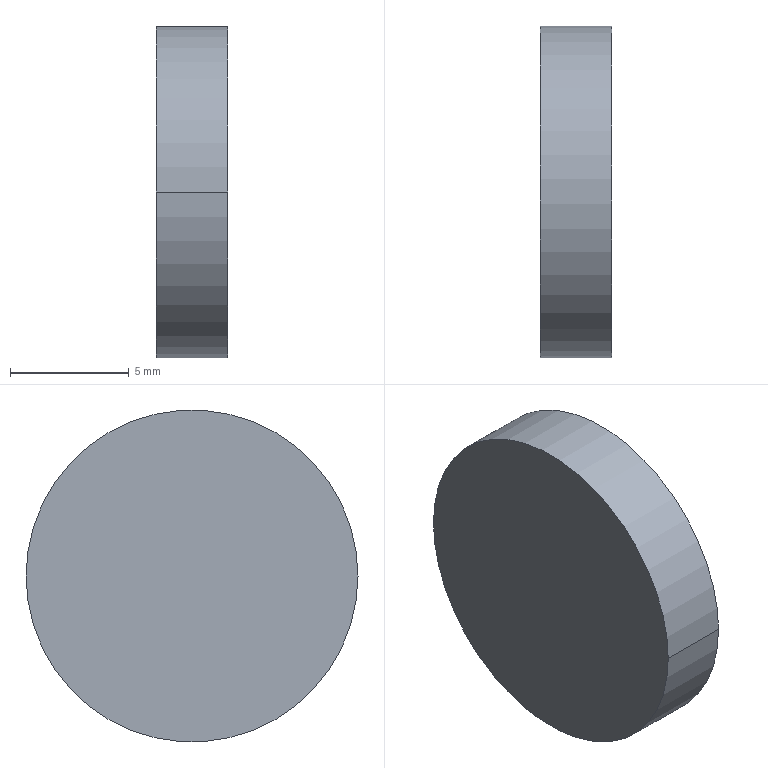Part | STEP file | LG-CAP_M8 | 1 solid | 4 faces | box 3 x 14 x 14 mm | volume 461.814 mm3 | cylinder 2 | plane 2 | commonest cylinder face diameters 14 x2
STEP:
#1=CARTESIAN_POINT('',(0.,0.,0.));
#2=DIRECTION('',(0.,0.,1.));
#3=DIRECTION('',(1.,0.,0.));
#4=AXIS2_PLACEMENT_3D('',#1,#2,#3);
#5=CARTESIAN_POINT('',(0.,-7.,0.));
#6=VERTEX_POINT('',#5);
#7=CARTESIAN_POINT('',(0.,7.,0.));
#8=VERTEX_POINT('',#7);
#9=CARTESIAN_POINT('',(0.,0.,0.));
#10=DIRECTION('',(1.,0.,0.));
#11=DIRECTION('',(0.,-1.,0.));
#12=AXIS2_PLACEMENT_3D('',#9,#10,#11);
#13=CIRCLE('',#12,7.);
#14=CARTESIAN_POINT('',(0.,0.,0.));
#15=DIRECTION('',(1.,0.,0.));
#16=DIRECTION('',(0.,-1.,0.));
#17=AXIS2_PLACEMENT_3D('',#14,#15,#16);
#18=CYLINDRICAL_SURFACE('',#17,7.);
#19=CARTESIAN_POINT('',(0.,0.));
#20=DIRECTION('',(1.,0.));
#21=VECTOR('',#20,1.);
#22=LINE('',#19,#21);
#23=(GEOMETRIC_REPRESENTATION_CONTEXT(2)PARAMETRIC_REPRESENTATION_CONTEXT()REPRESENTATION_CONTEXT('',''));
#24=DEFINITIONAL_REPRESENTATION('',(#22),#23);
#25=PCURVE('',#18,#24);
#26=CARTESIAN_POINT('',(0.,0.,0.));
#27=DIRECTION('',(-1.,0.,0.));
#28=DIRECTION('',(0.,1.,0.));
#29=AXIS2_PLACEMENT_3D('',#26,#27,#28);
#30=PLANE('',#29);
#31=CARTESIAN_POINT('',(-7.,0.));
#32=CARTESIAN_POINT('',(-7.,12.124));
#33=CARTESIAN_POINT('',(3.5,6.062));
#34=CARTESIAN_POINT('',(14.,0.));
#35=CARTESIAN_POINT('',(3.5,-6.062));
#36=CARTESIAN_POINT('',(-7.,-12.124));
#37=CARTESIAN_POINT('',(-7.,0.));
#38=(BOUNDED_CURVE()B_SPLINE_CURVE(2,(#31,#32,#33,#34,#35,#36,#37),.UNSPECIFIED.,.T.,.F.)B_SPLINE_CURVE_WITH_KNOTS((1,2,2,2,2,1),(-2.094,0.,2.094,4.189,6.283,8.378),.UNSPECIFIED.)CURVE()GEOMETRIC_REPRESENTATION_ITEM()RATIONAL_B_SPLINE_CURVE((1.,0.5,1.,0.5,1.,0.5,1.))REPRESENTATION_ITEM(''));
#39=(GEOMETRIC_REPRESENTATION_CONTEXT(2)PARAMETRIC_REPRESENTATION_CONTEXT()REPRESENTATION_CONTEXT('',''));
#40=DEFINITIONAL_REPRESENTATION('',(#38),#39);
#41=PCURVE('',#30,#40);
#42=SURFACE_CURVE('',#13,(#25,#41),.PCURVE_S1.);
#43=EDGE_CURVE('',#6,#8,#42,.T.);
#44=ORIENTED_EDGE('',*,*,#43,.T.);
#45=CARTESIAN_POINT('',(3.,7.,0.));
#46=VERTEX_POINT('',#45);
#47=CARTESIAN_POINT('',(0.,7.,0.));
#48=DIRECTION('',(1.,0.,0.));
#49=VECTOR('',#48,1.);
#50=LINE('',#47,#49);
#51=CARTESIAN_POINT('',(3.142,0.));
#52=DIRECTION('',(0.,1.));
#53=VECTOR('',#52,1.);
#54=LINE('',#51,#53);
#55=(GEOMETRIC_REPRESENTATION_CONTEXT(2)PARAMETRIC_REPRESENTATION_CONTEXT()REPRESENTATION_CONTEXT('',''));
#56=DEFINITIONAL_REPRESENTATION('',(#54),#55);
#57=PCURVE('',#18,#56);
#58=CARTESIAN_POINT('',(0.,0.,0.));
#59=DIRECTION('',(1.,0.,0.));
#60=DIRECTION('',(0.,-1.,0.));
#61=AXIS2_PLACEMENT_3D('',#58,#59,#60);
#62=CYLINDRICAL_SURFACE('',#61,7.);
#63=CARTESIAN_POINT('',(3.142,0.));
#64=DIRECTION('',(0.,1.));
#65=VECTOR('',#64,1.);
#66=LINE('',#63,#65);
#67=(GEOMETRIC_REPRESENTATION_CONTEXT(2)PARAMETRIC_REPRESENTATION_CONTEXT()REPRESENTATION_CONTEXT('',''));
#68=DEFINITIONAL_REPRESENTATION('',(#66),#67);
#69=PCURVE('',#62,#68);
#70=SURFACE_CURVE('',#50,(#57,#69),.PCURVE_S1.);
#71=EDGE_CURVE('',#8,#46,#70,.T.);
#72=ORIENTED_EDGE('',*,*,#71,.T.);
#73=CARTESIAN_POINT('',(3.,-7.,0.));
#74=VERTEX_POINT('',#73);
#75=CARTESIAN_POINT('',(3.,0.,0.));
#76=DIRECTION('',(-1.,0.,0.));
#77=DIRECTION('',(0.,1.,0.));
#78=AXIS2_PLACEMENT_3D('',#75,#76,#77);
#79=CIRCLE('',#78,7.);
#80=CARTESIAN_POINT('',(3.142,3.));
#81=DIRECTION('',(-1.,0.));
#82=VECTOR('',#81,1.);
#83=LINE('',#80,#82);
#84=(GEOMETRIC_REPRESENTATION_CONTEXT(2)PARAMETRIC_REPRESENTATION_CONTEXT()REPRESENTATION_CONTEXT('',''));
#85=DEFINITIONAL_REPRESENTATION('',(#83),#84);
#86=PCURVE('',#18,#85);
#87=CARTESIAN_POINT('',(3.,0.,0.));
#88=DIRECTION('',(1.,0.,0.));
#89=DIRECTION('',(0.,-1.,0.));
#90=AXIS2_PLACEMENT_3D('',#87,#88,#89);
#91=PLANE('',#90);
#92=CARTESIAN_POINT('',(-7.,0.));
#93=CARTESIAN_POINT('',(-7.,12.124));
#94=CARTESIAN_POINT('',(3.5,6.062));
#95=CARTESIAN_POINT('',(14.,0.));
#96=CARTESIAN_POINT('',(3.5,-6.062));
#97=CARTESIAN_POINT('',(-7.,-12.124));
#98=CARTESIAN_POINT('',(-7.,0.));
#99=(BOUNDED_CURVE()B_SPLINE_CURVE(2,(#92,#93,#94,#95,#96,#97,#98),.UNSPECIFIED.,.T.,.F.)B_SPLINE_CURVE_WITH_KNOTS((1,2,2,2,2,1),(-2.094,0.,2.094,4.189,6.283,8.378),.UNSPECIFIED.)CURVE()GEOMETRIC_REPRESENTATION_ITEM()RATIONAL_B_SPLINE_CURVE((1.,0.5,1.,0.5,1.,0.5,1.))REPRESENTATION_ITEM(''));
#100=(GEOMETRIC_REPRESENTATION_CONTEXT(2)PARAMETRIC_REPRESENTATION_CONTEXT()REPRESENTATION_CONTEXT('',''));
#101=DEFINITIONAL_REPRESENTATION('',(#99),#100);
#102=PCURVE('',#91,#101);
#103=SURFACE_CURVE('',#79,(#86,#102),.PCURVE_S1.);
#104=EDGE_CURVE('',#46,#74,#103,.T.);
#105=ORIENTED_EDGE('',*,*,#104,.T.);
#106=CARTESIAN_POINT('',(0.,-7.,0.));
#107=DIRECTION('',(1.,0.,0.));
#108=VECTOR('',#107,1.);
#109=LINE('',#106,#108);
#110=CARTESIAN_POINT('',(0.,0.));
#111=DIRECTION('',(0.,1.));
#112=VECTOR('',#111,1.);
#113=LINE('',#110,#112);
#114=(GEOMETRIC_REPRESENTATION_CONTEXT(2)PARAMETRIC_REPRESENTATION_CONTEXT()REPRESENTATION_CONTEXT('',''));
#115=DEFINITIONAL_REPRESENTATION('',(#113),#114);
#116=PCURVE('',#18,#115);
#117=CARTESIAN_POINT('',(6.283,0.));
#118=DIRECTION('',(0.,1.));
#119=VECTOR('',#118,1.);
#120=LINE('',#117,#119);
#121=(GEOMETRIC_REPRESENTATION_CONTEXT(2)PARAMETRIC_REPRESENTATION_CONTEXT()REPRESENTATION_CONTEXT('',''));
#122=DEFINITIONAL_REPRESENTATION('',(#120),#121);
#123=PCURVE('',#62,#122);
#124=SURFACE_CURVE('',#109,(#116,#123),.PCURVE_S1.);
#125=EDGE_CURVE('',#6,#74,#124,.T.);
#126=ORIENTED_EDGE('',*,*,#125,.F.);
#127=EDGE_LOOP('',(#44,#72,#105,#126));
#128=FACE_BOUND('',#127,.T.);
#129=ADVANCED_FACE('',(#128),#18,.T.);
#130=CARTESIAN_POINT('',(3.,0.,0.));
#131=DIRECTION('',(-1.,0.,0.));
#132=DIRECTION('',(0.,1.,0.));
#133=AXIS2_PLACEMENT_3D('',#130,#131,#132);
#134=CIRCLE('',#133,7.);
#135=CARTESIAN_POINT('',(-7.,0.));
#136=CARTESIAN_POINT('',(-7.,12.124));
#137=CARTESIAN_POINT('',(3.5,6.062));
#138=CARTESIAN_POINT('',(14.,0.));
#139=CARTESIAN_POINT('',(3.5,-6.062));
#140=CARTESIAN_POINT('',(-7.,-12.124));
#141=CARTESIAN_POINT('',(-7.,0.));
#142=(BOUNDED_CURVE()B_SPLINE_CURVE(2,(#135,#136,#137,#138,#139,#140,#141),.UNSPECIFIED.,.T.,.F.)B_SPLINE_CURVE_WITH_KNOTS((1,2,2,2,2,1),(-2.094,0.,2.094,4.189,6.283,8.378),.UNSPECIFIED.)CURVE()GEOMETRIC_REPRESENTATION_ITEM()RATIONAL_B_SPLINE_CURVE((1.,0.5,1.,0.5,1.,0.5,1.))REPRESENTATION_ITEM(''));
#143=(GEOMETRIC_REPRESENTATION_CONTEXT(2)PARAMETRIC_REPRESENTATION_CONTEXT()REPRESENTATION_CONTEXT('',''));
#144=DEFINITIONAL_REPRESENTATION('',(#142),#143);
#145=PCURVE('',#91,#144);
#146=CARTESIAN_POINT('',(9.425,3.));
#147=DIRECTION('',(-1.,0.));
#148=VECTOR('',#147,1.);
#149=LINE('',#146,#148);
#150=(GEOMETRIC_REPRESENTATION_CONTEXT(2)PARAMETRIC_REPRESENTATION_CONTEXT()REPRESENTATION_CONTEXT('',''));
#151=DEFINITIONAL_REPRESENTATION('',(#149),#150);
#152=PCURVE('',#62,#151);
#153=SURFACE_CURVE('',#134,(#145,#152),.PCURVE_S1.);
#154=EDGE_CURVE('',#74,#46,#153,.T.);
#155=ORIENTED_EDGE('',*,*,#154,.F.);
#156=ORIENTED_EDGE('',*,*,#104,.F.);
#157=EDGE_LOOP('',(#155,#156));
#158=FACE_BOUND('',#157,.T.);
#159=ADVANCED_FACE('',(#158),#91,.T.);
#160=ORIENTED_EDGE('',*,*,#43,.F.);
#161=CARTESIAN_POINT('',(0.,0.,0.));
#162=DIRECTION('',(1.,0.,0.));
#163=DIRECTION('',(0.,-1.,0.));
#164=AXIS2_PLACEMENT_3D('',#161,#162,#163);
#165=CIRCLE('',#164,7.);
#166=CARTESIAN_POINT('',(-7.,0.));
#167=CARTESIAN_POINT('',(-7.,12.124));
#168=CARTESIAN_POINT('',(3.5,6.062));
#169=CARTESIAN_POINT('',(14.,0.));
#170=CARTESIAN_POINT('',(3.5,-6.062));
#171=CARTESIAN_POINT('',(-7.,-12.124));
#172=CARTESIAN_POINT('',(-7.,0.));
#173=(BOUNDED_CURVE()B_SPLINE_CURVE(2,(#166,#167,#168,#169,#170,#171,#172),.UNSPECIFIED.,.T.,.F.)B_SPLINE_CURVE_WITH_KNOTS((1,2,2,2,2,1),(-2.094,0.,2.094,4.189,6.283,8.378),.UNSPECIFIED.)CURVE()GEOMETRIC_REPRESENTATION_ITEM()RATIONAL_B_SPLINE_CURVE((1.,0.5,1.,0.5,1.,0.5,1.))REPRESENTATION_ITEM(''));
#174=(GEOMETRIC_REPRESENTATION_CONTEXT(2)PARAMETRIC_REPRESENTATION_CONTEXT()REPRESENTATION_CONTEXT('',''));
#175=DEFINITIONAL_REPRESENTATION('',(#173),#174);
#176=PCURVE('',#30,#175);
#177=CARTESIAN_POINT('',(0.,0.));
#178=DIRECTION('',(1.,0.));
#179=VECTOR('',#178,1.);
#180=LINE('',#177,#179);
#181=(GEOMETRIC_REPRESENTATION_CONTEXT(2)PARAMETRIC_REPRESENTATION_CONTEXT()REPRESENTATION_CONTEXT('',''));
#182=DEFINITIONAL_REPRESENTATION('',(#180),#181);
#183=PCURVE('',#62,#182);
#184=SURFACE_CURVE('',#165,(#176,#183),.PCURVE_S1.);
#185=EDGE_CURVE('',#8,#6,#184,.T.);
#186=ORIENTED_EDGE('',*,*,#185,.F.);
#187=EDGE_LOOP('',(#160,#186));
#188=FACE_BOUND('',#187,.T.);
#189=ADVANCED_FACE('',(#188),#30,.T.);
#190=ORIENTED_EDGE('',*,*,#71,.F.);
#191=ORIENTED_EDGE('',*,*,#185,.T.);
#192=ORIENTED_EDGE('',*,*,#125,.T.);
#193=ORIENTED_EDGE('',*,*,#154,.T.);
#194=EDGE_LOOP('',(#190,#191,#192,#193));
#195=FACE_BOUND('',#194,.T.);
#196=ADVANCED_FACE('',(#195),#62,.T.);
#197=CLOSED_SHELL('',(#129,#159,#189,#196));
#198=MANIFOLD_SOLID_BREP('',#197);
#199=(LENGTH_UNIT()NAMED_UNIT(*)SI_UNIT(.MILLI.,.METRE.));
#200=UNCERTAINTY_MEASURE_WITH_UNIT(LENGTH_MEASURE(0.0000001),#199,'','');
#201=(NAMED_UNIT(*)PLANE_ANGLE_UNIT()SI_UNIT($,.RADIAN.));
#202=(NAMED_UNIT(*)SI_UNIT($,.STERADIAN.)SOLID_ANGLE_UNIT());
#203=(GEOMETRIC_REPRESENTATION_CONTEXT(3)GLOBAL_UNCERTAINTY_ASSIGNED_CONTEXT((#200))GLOBAL_UNIT_ASSIGNED_CONTEXT((#199,#201,#202))REPRESENTATION_CONTEXT('',''));
#204=ADVANCED_BREP_SHAPE_REPRESENTATION('',(#4,#198),#203);